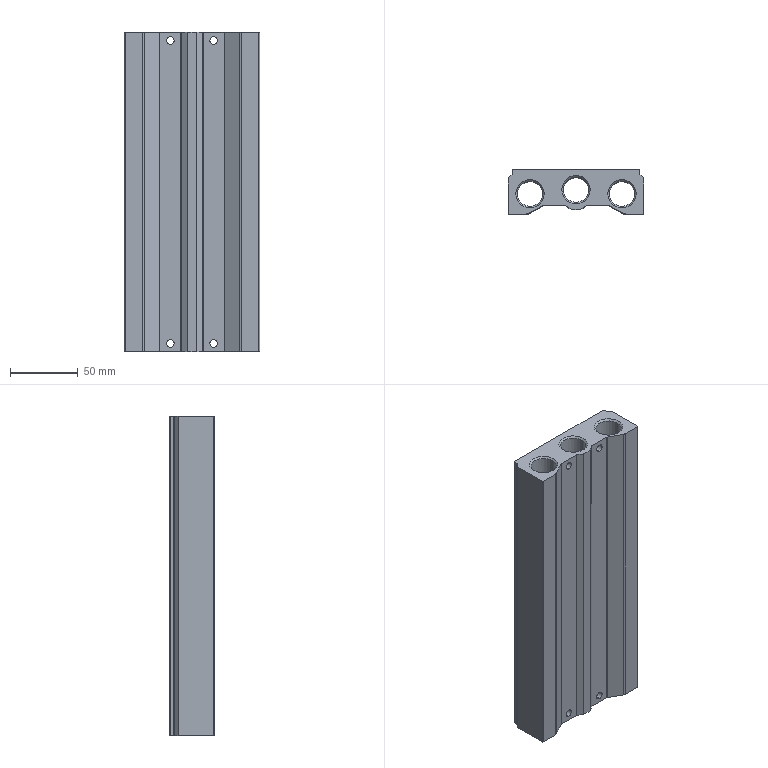Part | SolidWorks | features BaseBody 1 | 1 solid | 166 faces | box 100 x 33 x 236 mm | volume 472074 mm3 | cylinder 88 | cone 60 | plane 18 | commonest cylinder face diameters 3.242 x24 12 x24 1 x12 14.5 x12 5.5 x8 18.631 x6